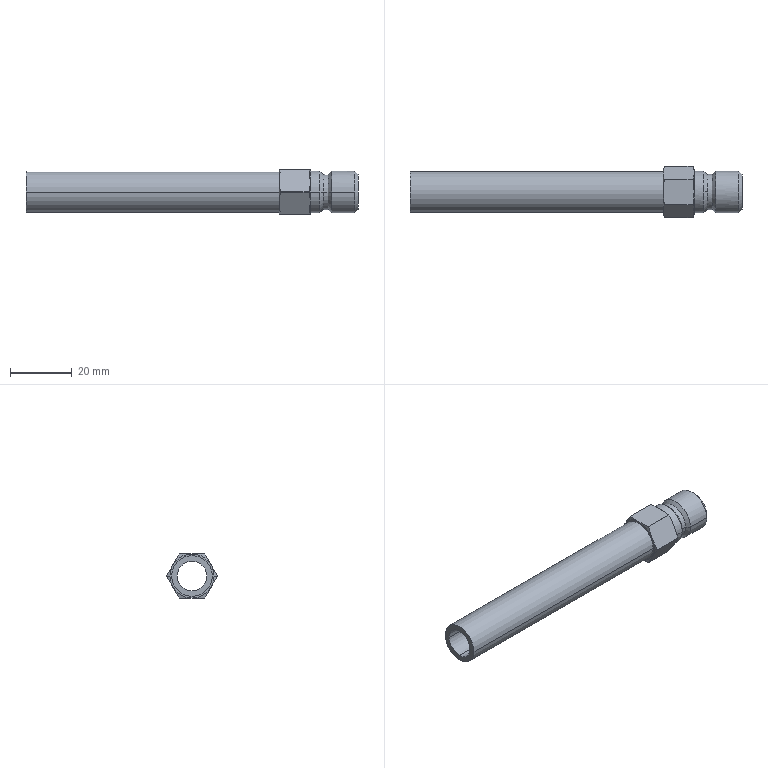Part | STEP file | 4-20.sldasm-Part-386 | 1 solid | 50 faces | box 107.317 x 16.497 x 14.3 mm | volume 7326 mm3 | cylinder 23 | cone 15 | plane 12 | commonest cylinder face diameters 16.497 x8 13.513 x6 9.525 x3 11.351 x3 13.157 x3